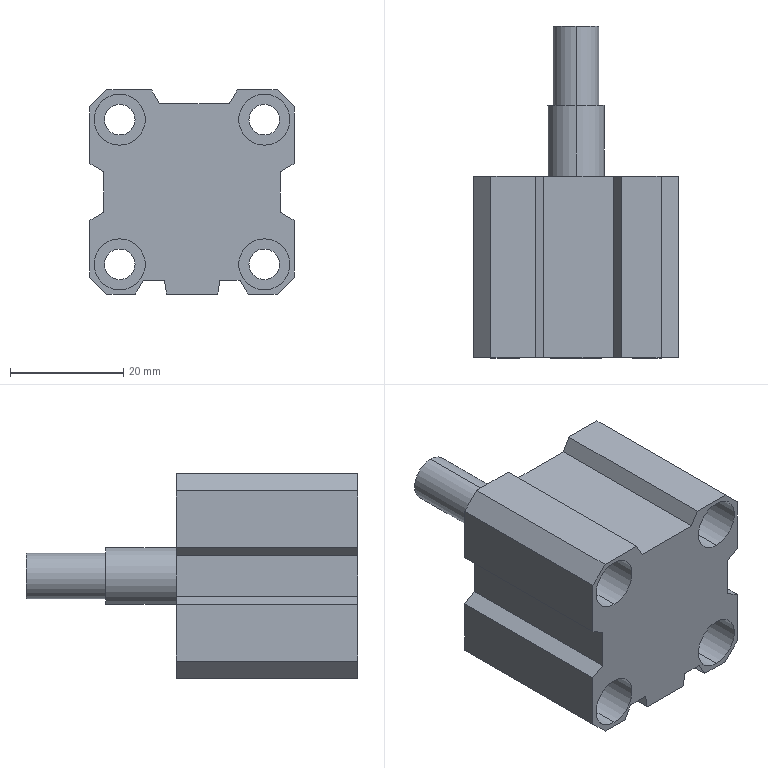Part | NX | 1 solid | 76 faces | box 36 x 58.5 x 36 mm | volume 33841 mm3 | plane 40 | cylinder 32 | cone 4 | commonest cylinder face diameters 9 x16 5.4 x8 4.5 x4 8 x2 10 x2